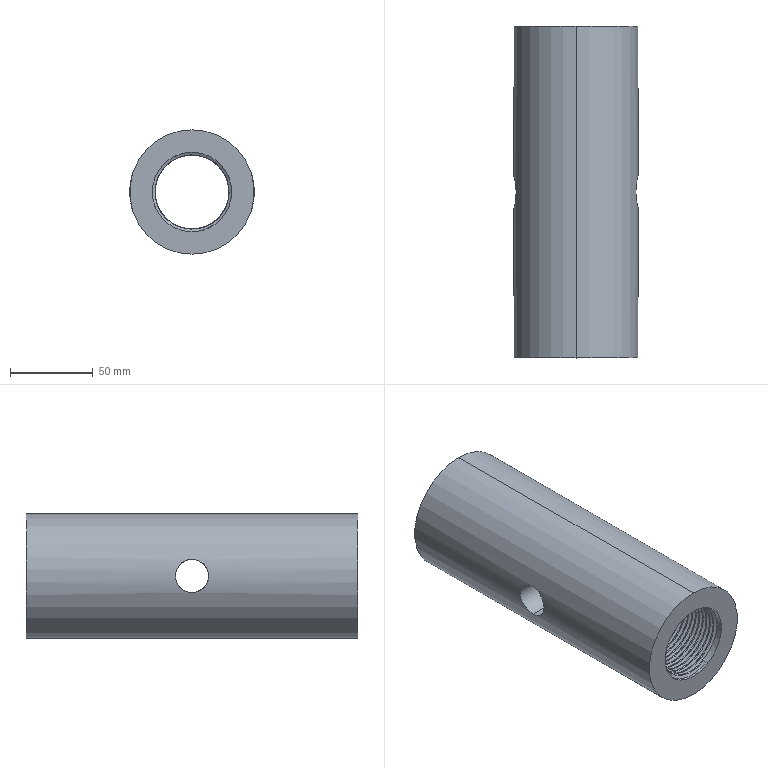Part | SolidWorks | features ICE 2, Extrusion 1, SweepThread 1 | 1 solid | 192 faces | box 75 x 200 x 75 mm | volume 538501 mm3 | cylinder 146 | spline 42 | plane 4 | commonest cylinder face diameters 48 x140 20 x4 75 x2